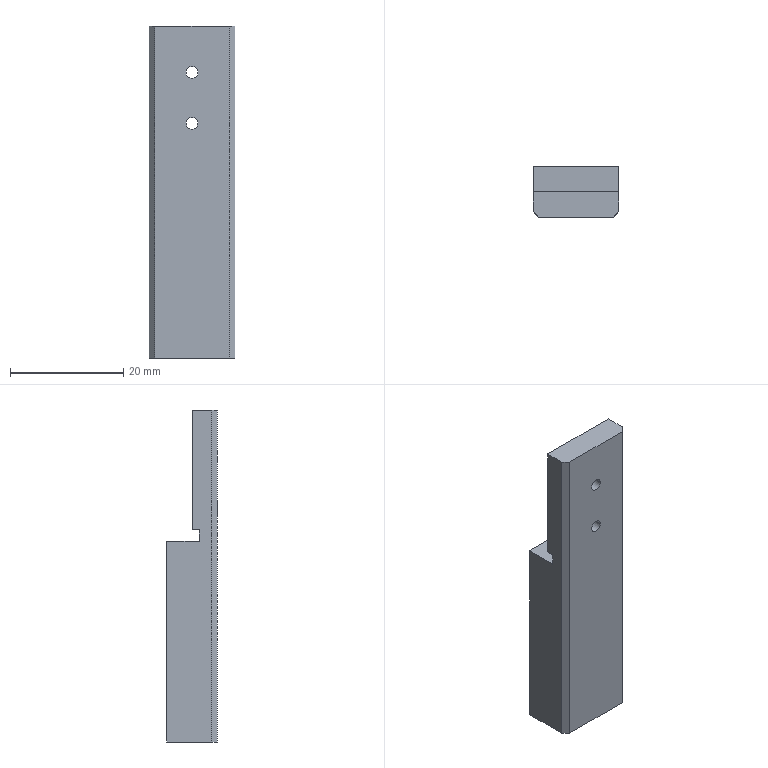Part | NX | 1 solid | 32 faces | box 15.2 x 9 x 58.7 mm | volume 6096 mm3 | plane 12 | cone 12 | cylinder 8 | commonest cylinder face diameters 2.1 x4 3.3 x4
STEP:
#1=CARTESIAN_POINT('',(15.2,4.5,37.5));
#2=VERTEX_POINT('',#1);
#3=CARTESIAN_POINT('',(0.,4.5,37.5));
#4=VERTEX_POINT('',#3);
#5=CARTESIAN_POINT('',(0.,4.5,37.5));
#6=DIRECTION('',(-1.,0.,0.));
#7=VECTOR('',#6,1000.);
#8=LINE('',#5,#7);
#9=EDGE_CURVE('',#2,#4,#8,.T.);
#10=ORIENTED_EDGE('',*,*,#9,.T.);
#11=CARTESIAN_POINT('',(0.,4.5,58.7));
#12=VERTEX_POINT('',#11);
#13=CARTESIAN_POINT('',(0.,4.5,0.));
#14=DIRECTION('',(0.,0.,-1.));
#15=VECTOR('',#14,1000.);
#16=LINE('',#13,#15);
#17=EDGE_CURVE('',#12,#4,#16,.T.);
#18=ORIENTED_EDGE('',*,*,#17,.F.);
#19=CARTESIAN_POINT('',(15.2,4.5,58.7));
#20=VERTEX_POINT('',#19);
#21=CARTESIAN_POINT('',(0.,4.5,58.7));
#22=DIRECTION('',(1.,0.,0.));
#23=VECTOR('',#22,1000.);
#24=LINE('',#21,#23);
#25=EDGE_CURVE('',#12,#20,#24,.T.);
#26=ORIENTED_EDGE('',*,*,#25,.T.);
#27=CARTESIAN_POINT('',(15.2,4.5,0.));
#28=DIRECTION('',(0.,0.,1.));
#29=VECTOR('',#28,1000.);
#30=LINE('',#27,#29);
#31=EDGE_CURVE('',#2,#20,#30,.T.);
#32=ORIENTED_EDGE('',*,*,#31,.F.);
#33=EDGE_LOOP('',(#10,#18,#26,#32));
#34=FACE_BOUND('',#33,.T.);
#35=CARTESIAN_POINT('',(9.,4.5,41.5));
#36=VERTEX_POINT('',#35);
#37=CARTESIAN_POINT('',(6.2,4.5,41.5));
#38=VERTEX_POINT('',#37);
#39=CARTESIAN_POINT('',(7.6,4.5,41.5));
#40=DIRECTION('',(0.,1.,0.));
#41=DIRECTION('',(1.,0.,0.));
#42=AXIS2_PLACEMENT_3D('',#39,#40,#41);
#43=CIRCLE('',#42,1.4);
#44=EDGE_CURVE('',#36,#38,#43,.T.);
#45=ORIENTED_EDGE('',*,*,#44,.F.);
#46=CARTESIAN_POINT('',(7.6,4.5,41.5));
#47=DIRECTION('',(0.,1.,0.));
#48=DIRECTION('',(1.,0.,0.));
#49=AXIS2_PLACEMENT_3D('',#46,#47,#48);
#50=CIRCLE('',#49,1.4);
#51=EDGE_CURVE('',#38,#36,#50,.T.);
#52=ORIENTED_EDGE('',*,*,#51,.F.);
#53=EDGE_LOOP('',(#45,#52));
#54=FACE_BOUND('',#53,.T.);
#55=CARTESIAN_POINT('',(9.,4.5,50.5));
#56=VERTEX_POINT('',#55);
#57=CARTESIAN_POINT('',(6.2,4.5,50.5));
#58=VERTEX_POINT('',#57);
#59=CARTESIAN_POINT('',(7.6,4.5,50.5));
#60=DIRECTION('',(0.,1.,0.));
#61=DIRECTION('',(1.,0.,0.));
#62=AXIS2_PLACEMENT_3D('',#59,#60,#61);
#63=CIRCLE('',#62,1.4);
#64=EDGE_CURVE('',#56,#58,#63,.T.);
#65=ORIENTED_EDGE('',*,*,#64,.F.);
#66=CARTESIAN_POINT('',(7.6,4.5,50.5));
#67=DIRECTION('',(0.,1.,0.));
#68=DIRECTION('',(1.,0.,0.));
#69=AXIS2_PLACEMENT_3D('',#66,#67,#68);
#70=CIRCLE('',#69,1.4);
#71=EDGE_CURVE('',#58,#56,#70,.T.);
#72=ORIENTED_EDGE('',*,*,#71,.F.);
#73=EDGE_LOOP('',(#65,#72));
#74=FACE_BOUND('',#73,.T.);
#75=CARTESIAN_POINT('',(15.2,4.5,58.7));
#76=DIRECTION('',(0.,-1.,0.));
#77=DIRECTION('',(0.,0.,-1.));
#78=AXIS2_PLACEMENT_3D('',#75,#76,#77);
#79=PLANE('',#78);
#80=ADVANCED_FACE('',(#34,#54,#74),#79,.F.);
#81=CARTESIAN_POINT('',(14.2,0.,0.));
#82=VERTEX_POINT('',#81);
#83=CARTESIAN_POINT('',(1.,0.,0.));
#84=VERTEX_POINT('',#83);
#85=CARTESIAN_POINT('',(0.,0.,0.));
#86=DIRECTION('',(-1.,0.,0.));
#87=VECTOR('',#86,1000.);
#88=LINE('',#85,#87);
#89=EDGE_CURVE('',#82,#84,#88,.T.);
#90=ORIENTED_EDGE('',*,*,#89,.F.);
#91=CARTESIAN_POINT('',(14.2,0.,58.7));
#92=VERTEX_POINT('',#91);
#93=CARTESIAN_POINT('',(14.2,0.,58.7));
#94=DIRECTION('',(0.,0.,-1.));
#95=VECTOR('',#94,1000.);
#96=LINE('',#93,#95);
#97=EDGE_CURVE('',#92,#82,#96,.T.);
#98=ORIENTED_EDGE('',*,*,#97,.F.);
#99=CARTESIAN_POINT('',(1.,0.,58.7));
#100=VERTEX_POINT('',#99);
#101=CARTESIAN_POINT('',(0.,0.,58.7));
#102=DIRECTION('',(-1.,0.,0.));
#103=VECTOR('',#102,1000.);
#104=LINE('',#101,#103);
#105=EDGE_CURVE('',#92,#100,#104,.T.);
#106=ORIENTED_EDGE('',*,*,#105,.T.);
#107=CARTESIAN_POINT('',(1.,0.,58.7));
#108=DIRECTION('',(0.,0.,-1.));
#109=VECTOR('',#108,1000.);
#110=LINE('',#107,#109);
#111=EDGE_CURVE('',#100,#84,#110,.T.);
#112=ORIENTED_EDGE('',*,*,#111,.T.);
#113=EDGE_LOOP('',(#90,#98,#106,#112));
#114=FACE_BOUND('',#113,.T.);
#115=CARTESIAN_POINT('',(6.55,0.,41.5));
#116=VERTEX_POINT('',#115);
#117=CARTESIAN_POINT('',(8.65,0.,41.5));
#118=VERTEX_POINT('',#117);
#119=CARTESIAN_POINT('',(7.6,0.,41.5));
#120=DIRECTION('',(0.,1.,0.));
#121=DIRECTION('',(-1.,0.,0.));
#122=AXIS2_PLACEMENT_3D('',#119,#120,#121);
#123=CIRCLE('',#122,1.05);
#124=EDGE_CURVE('',#116,#118,#123,.T.);
#125=ORIENTED_EDGE('',*,*,#124,.T.);
#126=CARTESIAN_POINT('',(7.6,0.,41.5));
#127=DIRECTION('',(0.,1.,0.));
#128=DIRECTION('',(-1.,0.,0.));
#129=AXIS2_PLACEMENT_3D('',#126,#127,#128);
#130=CIRCLE('',#129,1.05);
#131=EDGE_CURVE('',#118,#116,#130,.T.);
#132=ORIENTED_EDGE('',*,*,#131,.T.);
#133=EDGE_LOOP('',(#125,#132));
#134=FACE_BOUND('',#133,.T.);
#135=CARTESIAN_POINT('',(8.65,0.,50.5));
#136=VERTEX_POINT('',#135);
#137=CARTESIAN_POINT('',(6.55,0.,50.5));
#138=VERTEX_POINT('',#137);
#139=CARTESIAN_POINT('',(7.6,0.,50.5));
#140=DIRECTION('',(0.,1.,0.));
#141=DIRECTION('',(-1.,0.,0.));
#142=AXIS2_PLACEMENT_3D('',#139,#140,#141);
#143=CIRCLE('',#142,1.05);
#144=EDGE_CURVE('',#136,#138,#143,.T.);
#145=ORIENTED_EDGE('',*,*,#144,.T.);
#146=CARTESIAN_POINT('',(7.6,0.,50.5));
#147=DIRECTION('',(0.,1.,0.));
#148=DIRECTION('',(-1.,0.,0.));
#149=AXIS2_PLACEMENT_3D('',#146,#147,#148);
#150=CIRCLE('',#149,1.05);
#151=EDGE_CURVE('',#138,#136,#150,.T.);
#152=ORIENTED_EDGE('',*,*,#151,.T.);
#153=EDGE_LOOP('',(#145,#152));
#154=FACE_BOUND('',#153,.T.);
#155=CARTESIAN_POINT('',(0.,0.,0.));
#156=DIRECTION('',(0.,-1.,0.));
#157=DIRECTION('',(0.,0.,-1.));
#158=AXIS2_PLACEMENT_3D('',#155,#156,#157);
#159=PLANE('',#158);
#160=ADVANCED_FACE('',(#114,#134,#154),#159,.T.);
#161=ORIENTED_EDGE('',*,*,#111,.F.);
#162=CARTESIAN_POINT('',(0.,1.,58.7));
#163=VERTEX_POINT('',#162);
#164=CARTESIAN_POINT('',(1.,0.,58.7));
#165=DIRECTION('',(-0.7071,0.7071,0.));
#166=VECTOR('',#165,1000.);
#167=LINE('',#164,#166);
#168=EDGE_CURVE('',#100,#163,#167,.T.);
#169=ORIENTED_EDGE('',*,*,#168,.T.);
#170=CARTESIAN_POINT('',(0.,1.,0.));
#171=VERTEX_POINT('',#170);
#172=CARTESIAN_POINT('',(0.,1.,0.));
#173=DIRECTION('',(0.,0.,-1.));
#174=VECTOR('',#173,1000.);
#175=LINE('',#172,#174);
#176=EDGE_CURVE('',#163,#171,#175,.T.);
#177=ORIENTED_EDGE('',*,*,#176,.T.);
#178=CARTESIAN_POINT('',(1.,0.,0.));
#179=DIRECTION('',(-0.7071,0.7071,0.));
#180=VECTOR('',#179,1000.);
#181=LINE('',#178,#180);
#182=EDGE_CURVE('',#84,#171,#181,.T.);
#183=ORIENTED_EDGE('',*,*,#182,.F.);
#184=EDGE_LOOP('',(#161,#169,#177,#183));
#185=FACE_BOUND('',#184,.T.);
#186=CARTESIAN_POINT('',(1.,0.,0.));
#187=DIRECTION('',(-0.7071,-0.7071,0.));
#188=DIRECTION('',(-0.7071,0.7071,0.));
#189=AXIS2_PLACEMENT_3D('',#186,#187,#188);
#190=PLANE('',#189);
#191=ADVANCED_FACE('',(#185),#190,.T.);
#192=CARTESIAN_POINT('',(0.,3.2,37.5));
#193=VERTEX_POINT('',#192);
#194=CARTESIAN_POINT('',(0.,0.,37.5));
#195=DIRECTION('',(0.,1.,0.));
#196=VECTOR('',#195,1000.);
#197=LINE('',#194,#196);
#198=EDGE_CURVE('',#193,#4,#197,.T.);
#199=ORIENTED_EDGE('',*,*,#198,.F.);
#200=CARTESIAN_POINT('',(0.,3.2,35.5));
#201=VERTEX_POINT('',#200);
#202=CARTESIAN_POINT('',(0.,3.2,0.));
#203=DIRECTION('',(0.,0.,1.));
#204=VECTOR('',#203,1000.);
#205=LINE('',#202,#204);
#206=EDGE_CURVE('',#201,#193,#205,.T.);
#207=ORIENTED_EDGE('',*,*,#206,.F.);
#208=CARTESIAN_POINT('',(0.,9.,35.5));
#209=VERTEX_POINT('',#208);
#210=CARTESIAN_POINT('',(0.,0.,35.5));
#211=DIRECTION('',(0.,-1.,0.));
#212=VECTOR('',#211,1000.);
#213=LINE('',#210,#212);
#214=EDGE_CURVE('',#209,#201,#213,.T.);
#215=ORIENTED_EDGE('',*,*,#214,.F.);
#216=CARTESIAN_POINT('',(0.,9.,0.));
#217=VERTEX_POINT('',#216);
#218=CARTESIAN_POINT('',(0.,9.,0.));
#219=DIRECTION('',(0.,0.,1.));
#220=VECTOR('',#219,1000.);
#221=LINE('',#218,#220);
#222=EDGE_CURVE('',#217,#209,#221,.T.);
#223=ORIENTED_EDGE('',*,*,#222,.F.);
#224=CARTESIAN_POINT('',(0.,0.,0.));
#225=DIRECTION('',(0.,-1.,0.));
#226=VECTOR('',#225,1000.);
#227=LINE('',#224,#226);
#228=EDGE_CURVE('',#217,#171,#227,.T.);
#229=ORIENTED_EDGE('',*,*,#228,.T.);
#230=ORIENTED_EDGE('',*,*,#176,.F.);
#231=CARTESIAN_POINT('',(0.,0.,58.7));
#232=DIRECTION('',(0.,-1.,0.));
#233=VECTOR('',#232,1000.);
#234=LINE('',#231,#233);
#235=EDGE_CURVE('',#12,#163,#234,.T.);
#236=ORIENTED_EDGE('',*,*,#235,.F.);
#237=ORIENTED_EDGE('',*,*,#17,.T.);
#238=EDGE_LOOP('',(#199,#207,#215,#223,#229,#230,#236,#237));
#239=FACE_BOUND('',#238,.T.);
#240=CARTESIAN_POINT('',(0.,9.,0.));
#241=DIRECTION('',(-1.,0.,0.));
#242=DIRECTION('',(0.,0.,1.));
#243=AXIS2_PLACEMENT_3D('',#240,#241,#242);
#244=PLANE('',#243);
#245=ADVANCED_FACE('',(#239),#244,.T.);
#246=CARTESIAN_POINT('',(15.2,3.2,37.5));
#247=VERTEX_POINT('',#246);
#248=CARTESIAN_POINT('',(15.2,0.,37.5));
#249=DIRECTION('',(0.,1.,0.));
#250=VECTOR('',#249,1000.);
#251=LINE('',#248,#250);
#252=EDGE_CURVE('',#247,#2,#251,.T.);
#253=ORIENTED_EDGE('',*,*,#252,.F.);
#254=CARTESIAN_POINT('',(0.,3.2,37.5));
#255=DIRECTION('',(1.,0.,0.));
#256=VECTOR('',#255,1000.);
#257=LINE('',#254,#256);
#258=EDGE_CURVE('',#193,#247,#257,.T.);
#259=ORIENTED_EDGE('',*,*,#258,.F.);
#260=ORIENTED_EDGE('',*,*,#198,.T.);
#261=ORIENTED_EDGE('',*,*,#9,.F.);
#262=EDGE_LOOP('',(#253,#259,#260,#261));
#263=FACE_BOUND('',#262,.T.);
#264=CARTESIAN_POINT('',(15.2,7.,37.5));
#265=DIRECTION('',(0.,0.,1.));
#266=DIRECTION('',(1.,0.,0.));
#267=AXIS2_PLACEMENT_3D('',#264,#265,#266);
#268=PLANE('',#267);
#269=ADVANCED_FACE('',(#263),#268,.F.);
#270=ORIENTED_EDGE('',*,*,#252,.T.);
#271=ORIENTED_EDGE('',*,*,#31,.T.);
#272=CARTESIAN_POINT('',(15.2,1.,58.7));
#273=VERTEX_POINT('',#272);
#274=CARTESIAN_POINT('',(15.2,0.,58.7));
#275=DIRECTION('',(0.,1.,0.));
#276=VECTOR('',#275,1000.);
#277=LINE('',#274,#276);
#278=EDGE_CURVE('',#273,#20,#277,.T.);
#279=ORIENTED_EDGE('',*,*,#278,.F.);
#280=CARTESIAN_POINT('',(15.2,1.,0.));
#281=VERTEX_POINT('',#280);
#282=CARTESIAN_POINT('',(15.2,1.,0.));
#283=DIRECTION('',(0.,0.,1.));
#284=VECTOR('',#283,1000.);
#285=LINE('',#282,#284);
#286=EDGE_CURVE('',#281,#273,#285,.T.);
#287=ORIENTED_EDGE('',*,*,#286,.F.);
#288=CARTESIAN_POINT('',(15.2,9.,0.));
#289=VERTEX_POINT('',#288);
#290=CARTESIAN_POINT('',(15.2,0.,0.));
#291=DIRECTION('',(0.,1.,0.));
#292=VECTOR('',#291,1000.);
#293=LINE('',#290,#292);
#294=EDGE_CURVE('',#281,#289,#293,.T.);
#295=ORIENTED_EDGE('',*,*,#294,.T.);
#296=CARTESIAN_POINT('',(15.2,9.,35.5));
#297=VERTEX_POINT('',#296);
#298=CARTESIAN_POINT('',(15.2,9.,0.));
#299=DIRECTION('',(0.,0.,-1.));
#300=VECTOR('',#299,1000.);
#301=LINE('',#298,#300);
#302=EDGE_CURVE('',#297,#289,#301,.T.);
#303=ORIENTED_EDGE('',*,*,#302,.F.);
#304=CARTESIAN_POINT('',(15.2,3.2,35.5));
#305=VERTEX_POINT('',#304);
#306=CARTESIAN_POINT('',(15.2,0.,35.5));
#307=DIRECTION('',(0.,1.,0.));
#308=VECTOR('',#307,1000.);
#309=LINE('',#306,#308);
#310=EDGE_CURVE('',#305,#297,#309,.T.);
#311=ORIENTED_EDGE('',*,*,#310,.F.);
#312=CARTESIAN_POINT('',(15.2,3.2,0.));
#313=DIRECTION('',(0.,0.,-1.));
#314=VECTOR('',#313,1000.);
#315=LINE('',#312,#314);
#316=EDGE_CURVE('',#247,#305,#315,.T.);
#317=ORIENTED_EDGE('',*,*,#316,.F.);
#318=EDGE_LOOP('',(#270,#271,#279,#287,#295,#303,#311,#317));
#319=FACE_BOUND('',#318,.T.);
#320=CARTESIAN_POINT('',(15.2,0.,0.));
#321=DIRECTION('',(1.,0.,0.));
#322=DIRECTION('',(0.,1.,0.));
#323=AXIS2_PLACEMENT_3D('',#320,#321,#322);
#324=PLANE('',#323);
#325=ADVANCED_FACE('',(#319),#324,.T.);
#326=ORIENTED_EDGE('',*,*,#316,.T.);
#327=CARTESIAN_POINT('',(0.,3.2,35.5));
#328=DIRECTION('',(1.,0.,0.));
#329=VECTOR('',#328,1000.);
#330=LINE('',#327,#329);
#331=EDGE_CURVE('',#201,#305,#330,.T.);
#332=ORIENTED_EDGE('',*,*,#331,.F.);
#333=ORIENTED_EDGE('',*,*,#206,.T.);
#334=ORIENTED_EDGE('',*,*,#258,.T.);
#335=EDGE_LOOP('',(#326,#332,#333,#334));
#336=FACE_BOUND('',#335,.T.);
#337=CARTESIAN_POINT('',(15.2,3.2,37.5));
#338=DIRECTION('',(0.,-1.,0.));
#339=DIRECTION('',(0.,0.,-1.));
#340=AXIS2_PLACEMENT_3D('',#337,#338,#339);
#341=PLANE('',#340);
#342=ADVANCED_FACE('',(#336),#341,.F.);
#343=ORIENTED_EDGE('',*,*,#310,.T.);
#344=CARTESIAN_POINT('',(0.,9.,35.5));
#345=DIRECTION('',(-1.,0.,0.));
#346=VECTOR('',#345,1000.);
#347=LINE('',#344,#346);
#348=EDGE_CURVE('',#297,#209,#347,.T.);
#349=ORIENTED_EDGE('',*,*,#348,.T.);
#350=ORIENTED_EDGE('',*,*,#214,.T.);
#351=ORIENTED_EDGE('',*,*,#331,.T.);
#352=EDGE_LOOP('',(#343,#349,#350,#351));
#353=FACE_BOUND('',#352,.T.);
#354=CARTESIAN_POINT('',(15.2,7.,35.5));
#355=DIRECTION('',(0.,0.,-1.));
#356=DIRECTION('',(0.,-1.,0.));
#357=AXIS2_PLACEMENT_3D('',#354,#355,#356);
#358=PLANE('',#357);
#359=ADVANCED_FACE('',(#353),#358,.F.);
#360=ORIENTED_EDGE('',*,*,#348,.F.);
#361=ORIENTED_EDGE('',*,*,#302,.T.);
#362=CARTESIAN_POINT('',(0.,9.,0.));
#363=DIRECTION('',(1.,0.,0.));
#364=VECTOR('',#363,1000.);
#365=LINE('',#362,#364);
#366=EDGE_CURVE('',#217,#289,#365,.T.);
#367=ORIENTED_EDGE('',*,*,#366,.F.);
#368=ORIENTED_EDGE('',*,*,#222,.T.);
#369=EDGE_LOOP('',(#360,#361,#367,#368));
#370=FACE_BOUND('',#369,.T.);
#371=CARTESIAN_POINT('',(15.2,9.,0.));
#372=DIRECTION('',(0.,1.,0.));
#373=DIRECTION('',(1.,0.,0.));
#374=AXIS2_PLACEMENT_3D('',#371,#372,#373);
#375=PLANE('',#374);
#376=ADVANCED_FACE('',(#370),#375,.T.);
#377=ORIENTED_EDGE('',*,*,#286,.T.);
#378=CARTESIAN_POINT('',(14.2,0.,58.7));
#379=DIRECTION('',(-0.7071,-0.7071,0.));
#380=VECTOR('',#379,1000.);
#381=LINE('',#378,#380);
#382=EDGE_CURVE('',#273,#92,#381,.T.);
#383=ORIENTED_EDGE('',*,*,#382,.T.);
#384=ORIENTED_EDGE('',*,*,#97,.T.);
#385=CARTESIAN_POINT('',(14.2,0.,0.));
#386=DIRECTION('',(-0.7071,-0.7071,0.));
#387=VECTOR('',#386,1000.);
#388=LINE('',#385,#387);
#389=EDGE_CURVE('',#281,#82,#388,.T.);
#390=ORIENTED_EDGE('',*,*,#389,.F.);
#391=EDGE_LOOP('',(#377,#383,#384,#390));
#392=FACE_BOUND('',#391,.T.);
#393=CARTESIAN_POINT('',(15.2,1.,0.));
#394=DIRECTION('',(0.7071,-0.7071,0.));
#395=DIRECTION('',(0.,0.,-1.));
#396=AXIS2_PLACEMENT_3D('',#393,#394,#395);
#397=PLANE('',#396);
#398=ADVANCED_FACE('',(#392),#397,.T.);
#399=ORIENTED_EDGE('',*,*,#25,.F.);
#400=ORIENTED_EDGE('',*,*,#235,.T.);
#401=ORIENTED_EDGE('',*,*,#168,.F.);
#402=ORIENTED_EDGE('',*,*,#105,.F.);
#403=ORIENTED_EDGE('',*,*,#382,.F.);
#404=ORIENTED_EDGE('',*,*,#278,.T.);
#405=EDGE_LOOP('',(#399,#400,#401,#402,#403,#404));
#406=FACE_BOUND('',#405,.T.);
#407=CARTESIAN_POINT('',(0.,0.,58.7));
#408=DIRECTION('',(0.,0.,1.));
#409=DIRECTION('',(1.,0.,0.));
#410=AXIS2_PLACEMENT_3D('',#407,#408,#409);
#411=PLANE('',#410);
#412=ADVANCED_FACE('',(#406),#411,.T.);
#413=ORIENTED_EDGE('',*,*,#89,.T.);
#414=ORIENTED_EDGE('',*,*,#182,.T.);
#415=ORIENTED_EDGE('',*,*,#228,.F.);
#416=ORIENTED_EDGE('',*,*,#366,.T.);
#417=ORIENTED_EDGE('',*,*,#294,.F.);
#418=ORIENTED_EDGE('',*,*,#389,.T.);
#419=EDGE_LOOP('',(#413,#414,#415,#416,#417,#418));
#420=FACE_BOUND('',#419,.T.);
#421=CARTESIAN_POINT('',(13.315,4.5,0.));
#422=VERTEX_POINT('',#421);
#423=CARTESIAN_POINT('',(8.685,4.5,0.));
#424=VERTEX_POINT('',#423);
#425=CARTESIAN_POINT('',(11.,4.5,0.));
#426=DIRECTION('',(0.,0.,-1.));
#427=DIRECTION('',(-1.,0.,0.));
#428=AXIS2_PLACEMENT_3D('',#425,#426,#427);
#429=CIRCLE('',#428,2.315);
#430=EDGE_CURVE('',#422,#424,#429,.T.);
#431=ORIENTED_EDGE('',*,*,#430,.F.);
#432=CARTESIAN_POINT('',(11.,4.5,0.));
#433=DIRECTION('',(0.,0.,-1.));
#434=DIRECTION('',(-1.,0.,0.));
#435=AXIS2_PLACEMENT_3D('',#432,#433,#434);
#436=CIRCLE('',#435,2.315);
#437=EDGE_CURVE('',#424,#422,#436,.T.);
#438=ORIENTED_EDGE('',*,*,#437,.F.);
#439=EDGE_LOOP('',(#431,#438));
#440=FACE_BOUND('',#439,.T.);
#441=CARTESIAN_POINT('',(5.315,4.5,0.));
#442=VERTEX_POINT('',#441);
#443=CARTESIAN_POINT('',(0.685,4.5,0.));
#444=VERTEX_POINT('',#443);
#445=CARTESIAN_POINT('',(3.,4.5,0.));
#446=DIRECTION('',(0.,0.,-1.));
#447=DIRECTION('',(-1.,0.,0.));
#448=AXIS2_PLACEMENT_3D('',#445,#446,#447);
#449=CIRCLE('',#448,2.315);
#450=EDGE_CURVE('',#442,#444,#449,.T.);
#451=ORIENTED_EDGE('',*,*,#450,.F.);
#452=CARTESIAN_POINT('',(3.,4.5,0.));
#453=DIRECTION('',(0.,0.,-1.));
#454=DIRECTION('',(-1.,0.,0.));
#455=AXIS2_PLACEMENT_3D('',#452,#453,#454);
#456=CIRCLE('',#455,2.315);
#457=EDGE_CURVE('',#444,#442,#456,.T.);
#458=ORIENTED_EDGE('',*,*,#457,.F.);
#459=EDGE_LOOP('',(#451,#458));
#460=FACE_BOUND('',#459,.T.);
#461=CARTESIAN_POINT('',(0.,0.,0.));
#462=DIRECTION('',(0.,0.,1.));
#463=DIRECTION('',(1.,0.,0.));
#464=AXIS2_PLACEMENT_3D('',#461,#462,#463);
#465=PLANE('',#464);
#466=ADVANCED_FACE('',(#420,#440,#460),#465,.F.);
#467=CARTESIAN_POINT('',(12.65,4.5,12.2));
#468=VERTEX_POINT('',#467);
#469=CARTESIAN_POINT('',(9.35,4.5,12.2));
#470=VERTEX_POINT('',#469);
#471=CARTESIAN_POINT('',(11.,4.5,12.2));
#472=DIRECTION('',(0.,0.,1.));
#473=DIRECTION('',(0.,1.,0.));
#474=AXIS2_PLACEMENT_3D('',#471,#472,#473);
#475=CIRCLE('',#474,1.65);
#476=EDGE_CURVE('',#468,#470,#475,.T.);
#477=ORIENTED_EDGE('',*,*,#476,.T.);
#478=CARTESIAN_POINT('',(9.35,4.5,0.3839));
#479=VERTEX_POINT('',#478);
#480=CARTESIAN_POINT('',(9.35,4.5,4.));
#481=DIRECTION('',(0.,0.,-1.));
#482=VECTOR('',#481,1000.);
#483=LINE('',#480,#482);
#484=EDGE_CURVE('',#479,#470,#483,.F.);
#485=ORIENTED_EDGE('',*,*,#484,.F.);
#486=CARTESIAN_POINT('',(12.65,4.5,0.3839));
#487=VERTEX_POINT('',#486);
#488=CARTESIAN_POINT('',(11.,4.5,0.3839));
#489=DIRECTION('',(0.,0.,-1.));
#490=DIRECTION('',(-1.,0.,0.));
#491=AXIS2_PLACEMENT_3D('',#488,#489,#490);
#492=CIRCLE('',#491,1.65);
#493=EDGE_CURVE('',#479,#487,#492,.T.);
#494=ORIENTED_EDGE('',*,*,#493,.T.);
#495=CARTESIAN_POINT('',(12.65,4.5,4.));
#496=DIRECTION('',(0.,0.,-1.));
#497=VECTOR('',#496,1000.);
#498=LINE('',#495,#497);
#499=EDGE_CURVE('',#487,#468,#498,.F.);
#500=ORIENTED_EDGE('',*,*,#499,.T.);
#501=EDGE_LOOP('',(#477,#485,#494,#500));
#502=FACE_BOUND('',#501,.T.);
#503=CARTESIAN_POINT('',(11.,4.5,4.));
#504=DIRECTION('',(0.,0.,-1.));
#505=DIRECTION('',(-1.,0.,0.));
#506=AXIS2_PLACEMENT_3D('',#503,#504,#505);
#507=CYLINDRICAL_SURFACE('',#506,1.65);
#508=ADVANCED_FACE('',(#502),#507,.F.);
#509=ORIENTED_EDGE('',*,*,#493,.F.);
#510=CARTESIAN_POINT('',(9.35,4.5,0.3839));
#511=DIRECTION('',(-0.866,0.,-0.5));
#512=VECTOR('',#511,1000.);
#513=LINE('',#510,#512);
#514=EDGE_CURVE('',#424,#479,#513,.F.);
#515=ORIENTED_EDGE('',*,*,#514,.F.);
#516=ORIENTED_EDGE('',*,*,#437,.T.);
#517=CARTESIAN_POINT('',(12.65,4.5,0.3839));
#518=DIRECTION('',(0.866,0.,-0.5));
#519=VECTOR('',#518,1000.);
#520=LINE('',#517,#519);
#521=EDGE_CURVE('',#422,#487,#520,.F.);
#522=ORIENTED_EDGE('',*,*,#521,.T.);
#523=EDGE_LOOP('',(#509,#515,#516,#522));
#524=FACE_BOUND('',#523,.T.);
#525=CARTESIAN_POINT('',(11.,4.5,0.3839));
#526=DIRECTION('',(0.,0.,-1.));
#527=DIRECTION('',(-1.,0.,0.));
#528=AXIS2_PLACEMENT_3D('',#525,#526,#527);
#529=CONICAL_SURFACE('',#528,1.65,1.047);
#530=ADVANCED_FACE('',(#524),#529,.F.);
#531=ORIENTED_EDGE('',*,*,#64,.T.);
#532=CARTESIAN_POINT('',(6.55,4.15,50.5));
#533=VERTEX_POINT('',#532);
#534=CARTESIAN_POINT('',(6.55,4.15,50.5));
#535=DIRECTION('',(-0.7071,0.7071,0.));
#536=VECTOR('',#535,1000.);
#537=LINE('',#534,#536);
#538=EDGE_CURVE('',#58,#533,#537,.F.);
#539=ORIENTED_EDGE('',*,*,#538,.T.);
#540=CARTESIAN_POINT('',(8.65,4.15,50.5));
#541=VERTEX_POINT('',#540);
#542=CARTESIAN_POINT('',(7.6,4.15,50.5));
#543=DIRECTION('',(0.,1.,0.));
#544=DIRECTION('',(1.,0.,0.));
#545=AXIS2_PLACEMENT_3D('',#542,#543,#544);
#546=CIRCLE('',#545,1.05);
#547=EDGE_CURVE('',#541,#533,#546,.T.);
#548=ORIENTED_EDGE('',*,*,#547,.F.);
#549=CARTESIAN_POINT('',(8.65,4.15,50.5));
#550=DIRECTION('',(0.7071,0.7071,0.));
#551=VECTOR('',#550,1000.);
#552=LINE('',#549,#551);
#553=EDGE_CURVE('',#56,#541,#552,.F.);
#554=ORIENTED_EDGE('',*,*,#553,.F.);
#555=EDGE_LOOP('',(#531,#539,#548,#554));
#556=FACE_BOUND('',#555,.T.);
#557=CARTESIAN_POINT('',(7.6,4.15,50.5));
#558=DIRECTION('',(0.,1.,0.));
#559=DIRECTION('',(1.,0.,0.));
#560=AXIS2_PLACEMENT_3D('',#557,#558,#559);
#561=CONICAL_SURFACE('',#560,1.05,0.7854);
#562=ADVANCED_FACE('',(#556),#561,.F.);
#563=CARTESIAN_POINT('',(11.,4.5,13.191));
#564=VERTEX_POINT('',#563);
#565=CARTESIAN_POINT('',(12.65,4.5,12.2));
#566=DIRECTION('',(0.8572,0.,-0.515));
#567=VECTOR('',#566,1000.);
#568=LINE('',#565,#567);
#569=EDGE_CURVE('',#564,#468,#568,.T.);
#570=ORIENTED_EDGE('',*,*,#569,.T.);
#571=CARTESIAN_POINT('',(11.,4.5,12.2));
#572=DIRECTION('',(0.,0.,1.));
#573=DIRECTION('',(0.,1.,0.));
#574=AXIS2_PLACEMENT_3D('',#571,#572,#573);
#575=CIRCLE('',#574,1.65);
#576=EDGE_CURVE('',#470,#468,#575,.T.);
#577=ORIENTED_EDGE('',*,*,#576,.F.);
#578=CARTESIAN_POINT('',(9.35,4.5,12.2));
#579=DIRECTION('',(-0.8572,0.,-0.515));
#580=VECTOR('',#579,1000.);
#581=LINE('',#578,#580);
#582=EDGE_CURVE('',#564,#470,#581,.T.);
#583=ORIENTED_EDGE('',*,*,#582,.F.);
#584=EDGE_LOOP('',(#570,#577,#583));
#585=FACE_BOUND('',#584,.T.);
#586=CARTESIAN_POINT('',(11.,4.5,12.2));
#587=DIRECTION('',(0.,0.,-1.));
#588=DIRECTION('',(-1.,0.,0.));
#589=AXIS2_PLACEMENT_3D('',#586,#587,#588);
#590=CONICAL_SURFACE('',#589,1.65,1.03);
#591=ADVANCED_FACE('',(#585),#590,.F.);
#592=CARTESIAN_POINT('',(6.55,4.15,41.5));
#593=VERTEX_POINT('',#592);
#594=CARTESIAN_POINT('',(8.65,4.15,41.5));
#595=VERTEX_POINT('',#594);
#596=CARTESIAN_POINT('',(7.6,4.15,41.5));
#597=DIRECTION('',(0.,1.,0.));
#598=DIRECTION('',(1.,0.,0.));
#599=AXIS2_PLACEMENT_3D('',#596,#597,#598);
#600=CIRCLE('',#599,1.05);
#601=EDGE_CURVE('',#593,#595,#600,.T.);
#602=ORIENTED_EDGE('',*,*,#601,.F.);
#603=CARTESIAN_POINT('',(6.55,4.15,41.5));
#604=DIRECTION('',(-0.7071,0.7071,0.));
#605=VECTOR('',#604,1000.);
#606=LINE('',#603,#605);
#607=EDGE_CURVE('',#38,#593,#606,.F.);
#608=ORIENTED_EDGE('',*,*,#607,.F.);
#609=ORIENTED_EDGE('',*,*,#51,.T.);
#610=CARTESIAN_POINT('',(8.65,4.15,41.5));
#611=DIRECTION('',(0.7071,0.7071,0.));
#612=VECTOR('',#611,1000.);
#613=LINE('',#610,#612);
#614=EDGE_CURVE('',#36,#595,#613,.F.);
#615=ORIENTED_EDGE('',*,*,#614,.T.);
#616=EDGE_LOOP('',(#602,#608,#609,#615));
#617=FACE_BOUND('',#616,.T.);
#618=CARTESIAN_POINT('',(7.6,4.15,41.5));
#619=DIRECTION('',(0.,1.,0.));
#620=DIRECTION('',(1.,0.,0.));
#621=AXIS2_PLACEMENT_3D('',#618,#619,#620);
#622=CONICAL_SURFACE('',#621,1.05,0.7854);
#623=ADVANCED_FACE('',(#617),#622,.F.);
#624=CARTESIAN_POINT('',(4.65,4.5,0.3839));
#625=VERTEX_POINT('',#624);
#626=CARTESIAN_POINT('',(1.35,4.5,0.3839));
#627=VERTEX_POINT('',#626);
#628=CARTESIAN_POINT('',(3.,4.5,0.3839));
#629=DIRECTION('',(0.,0.,-1.));
#630=DIRECTION('',(-1.,0.,0.));
#631=AXIS2_PLACEMENT_3D('',#628,#629,#630);
#632=CIRCLE('',#631,1.65);
#633=EDGE_CURVE('',#625,#627,#632,.T.);
#634=ORIENTED_EDGE('',*,*,#633,.F.);
#635=CARTESIAN_POINT('',(5.315,4.5,0.));
#636=DIRECTION('',(0.866,0.,-0.5));
#637=VECTOR('',#636,1000.);
#638=LINE('',#635,#637);
#639=EDGE_CURVE('',#442,#625,#638,.F.);
#640=ORIENTED_EDGE('',*,*,#639,.F.);
#641=ORIENTED_EDGE('',*,*,#450,.T.);
#642=CARTESIAN_POINT('',(0.685,4.5,0.));
#643=DIRECTION('',(-0.866,0.,-0.5));
#644=VECTOR('',#643,1000.);
#645=LINE('',#642,#644);
#646=EDGE_CURVE('',#444,#627,#645,.F.);
#647=ORIENTED_EDGE('',*,*,#646,.T.);
#648=EDGE_LOOP('',(#634,#640,#641,#647));
#649=FACE_BOUND('',#648,.T.);
#650=CARTESIAN_POINT('',(3.,4.5,0.));
#651=DIRECTION('',(0.,0.,-1.));
#652=DIRECTION('',(-1.,0.,0.));
#653=AXIS2_PLACEMENT_3D('',#650,#651,#652);
#654=CONICAL_SURFACE('',#653,2.315,1.047);
#655=ADVANCED_FACE('',(#649),#654,.F.);
#656=ORIENTED_EDGE('',*,*,#633,.T.);
#657=CARTESIAN_POINT('',(1.35,4.5,12.2));
#658=VERTEX_POINT('',#657);
#659=CARTESIAN_POINT('',(1.35,4.5,10.1));
#660=DIRECTION('',(0.,0.,-1.));
#661=VECTOR('',#660,1000.);
#662=LINE('',#659,#661);
#663=EDGE_CURVE('',#627,#658,#662,.F.);
#664=ORIENTED_EDGE('',*,*,#663,.T.);
#665=CARTESIAN_POINT('',(4.65,4.5,12.2));
#666=VERTEX_POINT('',#665);
#667=CARTESIAN_POINT('',(3.,4.5,12.2));
#668=DIRECTION('',(0.,0.,1.));
#669=DIRECTION('',(0.,1.,0.));
#670=AXIS2_PLACEMENT_3D('',#667,#668,#669);
#671=CIRCLE('',#670,1.65);
#672=EDGE_CURVE('',#658,#666,#671,.T.);
#673=ORIENTED_EDGE('',*,*,#672,.T.);
#674=CARTESIAN_POINT('',(4.65,4.5,10.1));
#675=DIRECTION('',(0.,0.,-1.));
#676=VECTOR('',#675,1000.);
#677=LINE('',#674,#676);
#678=EDGE_CURVE('',#625,#666,#677,.F.);
#679=ORIENTED_EDGE('',*,*,#678,.F.);
#680=EDGE_LOOP('',(#656,#664,#673,#679));
#681=FACE_BOUND('',#680,.T.);
#682=CARTESIAN_POINT('',(3.,4.5,10.1));
#683=DIRECTION('',(0.,0.,-1.));
#684=DIRECTION('',(-1.,0.,0.));
#685=AXIS2_PLACEMENT_3D('',#682,#683,#684);
#686=CYLINDRICAL_SURFACE('',#685,1.65);
#687=ADVANCED_FACE('',(#681),#686,.F.);
#688=CARTESIAN_POINT('',(3.,4.5,12.2));
#689=DIRECTION('',(0.,0.,1.));
#690=DIRECTION('',(0.,1.,0.));
#691=AXIS2_PLACEMENT_3D('',#688,#689,#690);
#692=CIRCLE('',#691,1.65);
#693=EDGE_CURVE('',#666,#658,#692,.T.);
#694=ORIENTED_EDGE('',*,*,#693,.F.);
#695=CARTESIAN_POINT('',(3.,4.5,13.191));
#696=VERTEX_POINT('',#695);
#697=CARTESIAN_POINT('',(4.65,4.5,12.2));
#698=DIRECTION('',(0.8572,0.,-0.515));
#699=VECTOR('',#698,1000.);
#700=LINE('',#697,#699);
#701=EDGE_CURVE('',#696,#666,#700,.T.);
#702=ORIENTED_EDGE('',*,*,#701,.F.);
#703=CARTESIAN_POINT('',(1.35,4.5,12.2));
#704=DIRECTION('',(-0.8572,0.,-0.515));
#705=VECTOR('',#704,1000.);
#706=LINE('',#703,#705);
#707=EDGE_CURVE('',#696,#658,#706,.T.);
#708=ORIENTED_EDGE('',*,*,#707,.T.);
#709=EDGE_LOOP('',(#694,#702,#708));
#710=FACE_BOUND('',#709,.T.);
#711=CARTESIAN_POINT('',(3.,4.5,12.2));
#712=DIRECTION('',(0.,0.,-1.));
#713=DIRECTION('',(-1.,0.,0.));
#714=AXIS2_PLACEMENT_3D('',#711,#712,#713);
#715=CONICAL_SURFACE('',#714,1.65,1.03);
#716=ADVANCED_FACE('',(#710),#715,.F.);
#717=ORIENTED_EDGE('',*,*,#124,.F.);
#718=CARTESIAN_POINT('',(6.55,-0.9,41.5));
#719=DIRECTION('',(0.,1.,0.));
#720=VECTOR('',#719,1000.);
#721=LINE('',#718,#720);
#722=EDGE_CURVE('',#593,#116,#721,.F.);
#723=ORIENTED_EDGE('',*,*,#722,.F.);
#724=ORIENTED_EDGE('',*,*,#601,.T.);
#725=CARTESIAN_POINT('',(8.65,-0.9,41.5));
#726=DIRECTION('',(0.,1.,0.));
#727=VECTOR('',#726,1000.);
#728=LINE('',#725,#727);
#729=EDGE_CURVE('',#595,#118,#728,.F.);
#730=ORIENTED_EDGE('',*,*,#729,.T.);
#731=EDGE_LOOP('',(#717,#723,#724,#730));
#732=FACE_BOUND('',#731,.T.);
#733=CARTESIAN_POINT('',(7.6,-0.9,41.5));
#734=DIRECTION('',(0.,1.,0.));
#735=DIRECTION('',(-1.,0.,0.));
#736=AXIS2_PLACEMENT_3D('',#733,#734,#735);
#737=CYLINDRICAL_SURFACE('',#736,1.05);
#738=ADVANCED_FACE('',(#732),#737,.F.);
#739=ORIENTED_EDGE('',*,*,#144,.F.);
#740=CARTESIAN_POINT('',(8.65,-0.9,50.5));
#741=DIRECTION('',(0.,1.,0.));
#742=VECTOR('',#741,1000.);
#743=LINE('',#740,#742);
#744=EDGE_CURVE('',#136,#541,#743,.T.);
#745=ORIENTED_EDGE('',*,*,#744,.T.);
#746=ORIENTED_EDGE('',*,*,#547,.T.);
#747=CARTESIAN_POINT('',(6.55,-0.9,50.5));
#748=DIRECTION('',(0.,1.,0.));
#749=VECTOR('',#748,1000.);
#750=LINE('',#747,#749);
#751=EDGE_CURVE('',#138,#533,#750,.T.);
#752=ORIENTED_EDGE('',*,*,#751,.F.);
#753=EDGE_LOOP('',(#739,#745,#746,#752));
#754=FACE_BOUND('',#753,.T.);
#755=CARTESIAN_POINT('',(7.6,-0.9,50.5));
#756=DIRECTION('',(0.,1.,0.));
#757=DIRECTION('',(-1.,0.,0.));
#758=AXIS2_PLACEMENT_3D('',#755,#756,#757);
#759=CYLINDRICAL_SURFACE('',#758,1.05);
#760=ADVANCED_FACE('',(#754),#759,.F.);
#761=ORIENTED_EDGE('',*,*,#430,.T.);
#762=ORIENTED_EDGE('',*,*,#514,.T.);
#763=CARTESIAN_POINT('',(11.,4.5,0.3839));
#764=DIRECTION('',(0.,0.,-1.));
#765=DIRECTION('',(-1.,0.,0.));
#766=AXIS2_PLACEMENT_3D('',#763,#764,#765);
#767=CIRCLE('',#766,1.65);
#768=EDGE_CURVE('',#487,#479,#767,.T.);
#769=ORIENTED_EDGE('',*,*,#768,.F.);
#770=ORIENTED_EDGE('',*,*,#521,.F.);
#771=EDGE_LOOP('',(#761,#762,#769,#770));
#772=FACE_BOUND('',#771,.T.);
#773=CARTESIAN_POINT('',(11.,4.5,0.3839));
#774=DIRECTION('',(0.,0.,-1.));
#775=DIRECTION('',(-1.,0.,0.));
#776=AXIS2_PLACEMENT_3D('',#773,#774,#775);
#777=CONICAL_SURFACE('',#776,1.65,1.047);
#778=ADVANCED_FACE('',(#772),#777,.F.);
#779=ORIENTED_EDGE('',*,*,#44,.T.);
#780=ORIENTED_EDGE('',*,*,#607,.T.);
#781=CARTESIAN_POINT('',(7.6,4.15,41.5));
#782=DIRECTION('',(0.,1.,0.));
#783=DIRECTION('',(1.,0.,0.));
#784=AXIS2_PLACEMENT_3D('',#781,#782,#783);
#785=CIRCLE('',#784,1.05);
#786=EDGE_CURVE('',#595,#593,#785,.T.);
#787=ORIENTED_EDGE('',*,*,#786,.F.);
#788=ORIENTED_EDGE('',*,*,#614,.F.);
#789=EDGE_LOOP('',(#779,#780,#787,#788));
#790=FACE_BOUND('',#789,.T.);
#791=CARTESIAN_POINT('',(7.6,4.15,41.5));
#792=DIRECTION('',(0.,1.,0.));
#793=DIRECTION('',(1.,0.,0.));
#794=AXIS2_PLACEMENT_3D('',#791,#792,#793);
#795=CONICAL_SURFACE('',#794,1.05,0.7854);
#796=ADVANCED_FACE('',(#790),#795,.F.);
#797=ORIENTED_EDGE('',*,*,#693,.T.);
#798=ORIENTED_EDGE('',*,*,#663,.F.);
#799=CARTESIAN_POINT('',(3.,4.5,0.3839));
#800=DIRECTION('',(0.,0.,-1.));
#801=DIRECTION('',(-1.,0.,0.));
#802=AXIS2_PLACEMENT_3D('',#799,#800,#801);
#803=CIRCLE('',#802,1.65);
#804=EDGE_CURVE('',#627,#625,#803,.T.);
#805=ORIENTED_EDGE('',*,*,#804,.T.);
#806=ORIENTED_EDGE('',*,*,#678,.T.);
#807=EDGE_LOOP('',(#797,#798,#805,#806));
#808=FACE_BOUND('',#807,.T.);
#809=CARTESIAN_POINT('',(3.,4.5,10.1));
#810=DIRECTION('',(0.,0.,-1.));
#811=DIRECTION('',(-1.,0.,0.));
#812=AXIS2_PLACEMENT_3D('',#809,#810,#811);
#813=CYLINDRICAL_SURFACE('',#812,1.65);
#814=ADVANCED_FACE('',(#808),#813,.F.);
#815=ORIENTED_EDGE('',*,*,#484,.T.);
#816=ORIENTED_EDGE('',*,*,#576,.T.);
#817=ORIENTED_EDGE('',*,*,#499,.F.);
#818=ORIENTED_EDGE('',*,*,#768,.T.);
#819=EDGE_LOOP('',(#815,#816,#817,#818));
#820=FACE_BOUND('',#819,.T.);
#821=CARTESIAN_POINT('',(11.,4.5,4.));
#822=DIRECTION('',(0.,0.,-1.));
#823=DIRECTION('',(-1.,0.,0.));
#824=AXIS2_PLACEMENT_3D('',#821,#822,#823);
#825=CYLINDRICAL_SURFACE('',#824,1.65);
#826=ADVANCED_FACE('',(#820),#825,.F.);
#827=CARTESIAN_POINT('',(7.6,4.15,50.5));
#828=DIRECTION('',(0.,1.,0.));
#829=DIRECTION('',(1.,0.,0.));
#830=AXIS2_PLACEMENT_3D('',#827,#828,#829);
#831=CIRCLE('',#830,1.05);
#832=EDGE_CURVE('',#533,#541,#831,.T.);
#833=ORIENTED_EDGE('',*,*,#832,.T.);
#834=ORIENTED_EDGE('',*,*,#744,.F.);
#835=ORIENTED_EDGE('',*,*,#151,.F.);
#836=ORIENTED_EDGE('',*,*,#751,.T.);
#837=EDGE_LOOP('',(#833,#834,#835,#836));
#838=FACE_BOUND('',#837,.T.);
#839=CARTESIAN_POINT('',(7.6,-0.9,50.5));
#840=DIRECTION('',(0.,1.,0.));
#841=DIRECTION('',(-1.,0.,0.));
#842=AXIS2_PLACEMENT_3D('',#839,#840,#841);
#843=CYLINDRICAL_SURFACE('',#842,1.05);
#844=ADVANCED_FACE('',(#838),#843,.F.);
#845=ORIENTED_EDGE('',*,*,#701,.T.);
#846=ORIENTED_EDGE('',*,*,#672,.F.);
#847=ORIENTED_EDGE('',*,*,#707,.F.);
#848=EDGE_LOOP('',(#845,#846,#847));
#849=FACE_BOUND('',#848,.T.);
#850=CARTESIAN_POINT('',(3.,4.5,12.2));
#851=DIRECTION('',(0.,0.,-1.));
#852=DIRECTION('',(-1.,0.,0.));
#853=AXIS2_PLACEMENT_3D('',#850,#851,#852);
#854=CONICAL_SURFACE('',#853,1.65,1.03);
#855=ADVANCED_FACE('',(#849),#854,.F.);
#856=ORIENTED_EDGE('',*,*,#476,.F.);
#857=ORIENTED_EDGE('',*,*,#569,.F.);
#858=ORIENTED_EDGE('',*,*,#582,.T.);
#859=EDGE_LOOP('',(#856,#857,#858));
#860=FACE_BOUND('',#859,.T.);
#861=CARTESIAN_POINT('',(11.,4.5,12.2));
#862=DIRECTION('',(0.,0.,-1.));
#863=DIRECTION('',(-1.,0.,0.));
#864=AXIS2_PLACEMENT_3D('',#861,#862,#863);
#865=CONICAL_SURFACE('',#864,1.65,1.03);
#866=ADVANCED_FACE('',(#860),#865,.F.);
#867=ORIENTED_EDGE('',*,*,#832,.F.);
#868=ORIENTED_EDGE('',*,*,#538,.F.);
#869=ORIENTED_EDGE('',*,*,#71,.T.);
#870=ORIENTED_EDGE('',*,*,#553,.T.);
#871=EDGE_LOOP('',(#867,#868,#869,#870));
#872=FACE_BOUND('',#871,.T.);
#873=CARTESIAN_POINT('',(7.6,4.15,50.5));
#874=DIRECTION('',(0.,1.,0.));
#875=DIRECTION('',(1.,0.,0.));
#876=AXIS2_PLACEMENT_3D('',#873,#874,#875);
#877=CONICAL_SURFACE('',#876,1.05,0.7854);
#878=ADVANCED_FACE('',(#872),#877,.F.);
#879=ORIENTED_EDGE('',*,*,#722,.T.);
#880=ORIENTED_EDGE('',*,*,#131,.F.);
#881=ORIENTED_EDGE('',*,*,#729,.F.);
#882=ORIENTED_EDGE('',*,*,#786,.T.);
#883=EDGE_LOOP('',(#879,#880,#881,#882));
#884=FACE_BOUND('',#883,.T.);
#885=CARTESIAN_POINT('',(7.6,-0.9,41.5));
#886=DIRECTION('',(0.,1.,0.));
#887=DIRECTION('',(-1.,0.,0.));
#888=AXIS2_PLACEMENT_3D('',#885,#886,#887);
#889=CYLINDRICAL_SURFACE('',#888,1.05);
#890=ADVANCED_FACE('',(#884),#889,.F.);
#891=ORIENTED_EDGE('',*,*,#646,.F.);
#892=ORIENTED_EDGE('',*,*,#457,.T.);
#893=ORIENTED_EDGE('',*,*,#639,.T.);
#894=ORIENTED_EDGE('',*,*,#804,.F.);
#895=EDGE_LOOP('',(#891,#892,#893,#894));
#896=FACE_BOUND('',#895,.T.);
#897=CARTESIAN_POINT('',(3.,4.5,0.));
#898=DIRECTION('',(0.,0.,-1.));
#899=DIRECTION('',(-1.,0.,0.));
#900=AXIS2_PLACEMENT_3D('',#897,#898,#899);
#901=CONICAL_SURFACE('',#900,2.315,1.047);
#902=ADVANCED_FACE('',(#896),#901,.F.);
#903=CLOSED_SHELL('',(#80,#160,#191,#245,#269,#325,#342,#359,#376,#398,#412,#466,#508,#530,#562,#591,#623,#655,#687,#716,#738,#760,#778,#796,#814,#826,#844,#855,#866,#878,#890,#902));
#904=MANIFOLD_SOLID_BREP('',#903);
#905=(LENGTH_UNIT()NAMED_UNIT(*)SI_UNIT(.MILLI.,.METRE.));
#906=UNCERTAINTY_MEASURE_WITH_UNIT(LENGTH_MEASURE(0.00001),#905,'','');
#907=(NAMED_UNIT(*)PLANE_ANGLE_UNIT()SI_UNIT($,.RADIAN.));
#908=(NAMED_UNIT(*)SI_UNIT($,.STERADIAN.)SOLID_ANGLE_UNIT());
#909=(GEOMETRIC_REPRESENTATION_CONTEXT(3)GLOBAL_UNCERTAINTY_ASSIGNED_CONTEXT((#906))GLOBAL_UNIT_ASSIGNED_CONTEXT((#905,#907,#908))REPRESENTATION_CONTEXT('',''));
#910=ADVANCED_BREP_SHAPE_REPRESENTATION('',(#904),#909);